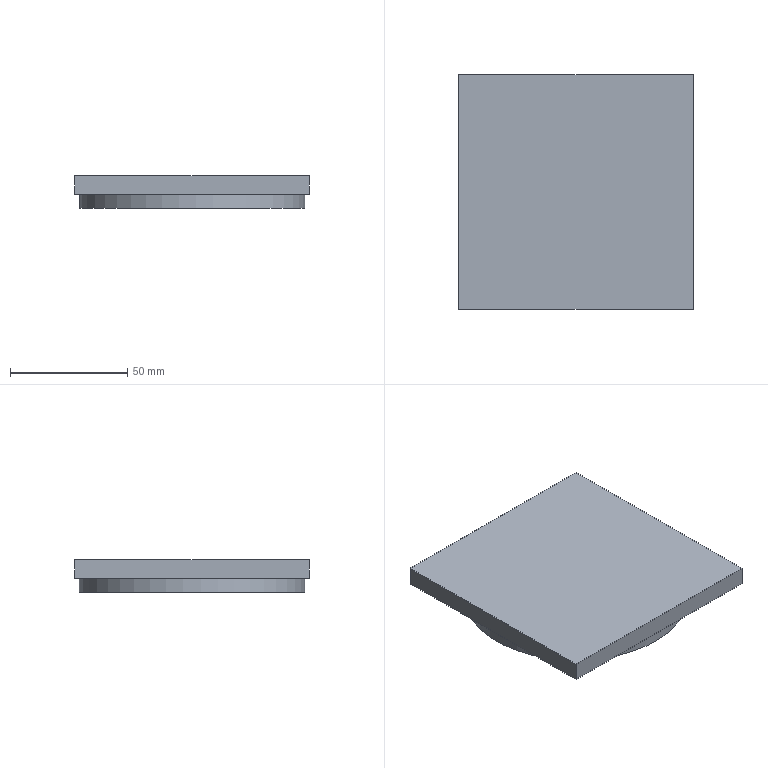NC program | NX | posted with a generic post | part box 100 x 100 x 14 mm
Whole program:
N10 G17 G21 G94 G90
(ADAPTIVE_MILLING_1_COPY , TOOL : D-12)
N12 T02 M6
N14 G54
N16 G17 G0 G90 X-1.135 Y5.279 S6000 M3
N18 G43 Z15. H2
N20 Z10.
N22 G94 G3 X-1.135 Y5.279 Z9.408 I1.135 J-5.279 F4000.
N24 X-1.135 Y5.279 Z8.816 I1.135 J-5.279
N26 X-1.135 Y5.279 Z8.223 I1.135 J-5.279
N28 X-1.135 Y5.279 Z7.631 I1.135 J-5.279
N30 X-1.135 Y5.279 Z7.039 I1.135 J-5.279
N32 X-1.135 Y5.279 Z6.447 I1.135 J-5.279
N34 X-1.135 Y5.279 Z5.854 I1.135 J-5.279
N36 X-1.135 Y5.279 Z5.262 I1.135 J-5.279
N38 X-1.135 Y5.279 Z4.67 I1.135 J-5.279
N40 X-1.135 Y5.279 Z4.078 I1.135 J-5.279
N42 X-1.135 Y5.279 Z3.485 I1.135 J-5.279
N44 X-1.135 Y5.279 Z2.893 I1.135 J-5.279
N46 X-1.135 Y5.279 Z2.301 I1.135 J-5.279
N48 X-1.135 Y5.279 Z1.709 I1.135 J-5.279
N50 X-1.135 Y5.279 Z1.116 I1.135 J-5.279
N52 X-1.135 Y5.279 Z0.524 I1.135 J-5.279
N54 X5.4 Y0. Z0.1 R-5.4
N56 X-3.183 Y-4.438 R-5.43
N58 X4.389 Y-3.32 R5.53
N60 X1.157 Y6.066 R5.7
N62 X0.068 Y-6.24 R-6.208
N64 X6.049 Y3.109 R6.703
N66 X-3.005 Y6.328 R6.76
N68 X-6.34 Y-3.048 R7.037
N70 X3.016 Y-6.393 R7.037
N72 X5.74 Y5.139 R7.442
N74 X-6.46 Y4.501 R7.722
N76 X2.461 Y-7.537 R7.902
N78 X0.478 Y8.702 R8.313
N80 X-6.031 Y-6.413 R8.751
N82 X6.609 Y-6.044 R9.029
N84 X0.165 Y9.64 R9.24
N86 X-7.235 Y-6.519 R9.676
N88 X6.659 Y-7.298 R9.937
N90 X1.171 Y10.532 R10.195
N92 X-9.22 Y-5.439 R10.635
N94 X5.817 Y-9.13 R10.861
N96 X1.397 Y11.498 R11.182
N98 X-10.325 Y-5.513 R11.627
N100 X5.527 Y-10.446 R11.852
N102 X2.228 Y12.392 R12.19
N104 X-11.976 Y-4.291 R12.627
N106 X4.618 Y-11.968 R12.843
N108 X6.27 Y12.045 R13.211
N110 X-11.992 Y6.715 R13.584
N112 X1.416 Y-13.769 R13.807
N114 X11.223 Y9.224 R14.234
N116 X-8.738 Y11.93 R14.517
N118 X-3.044 Y-14.576 R14.837
N120 X14.858 Y4.283 R15.27
N122 X-7.311 Y14.089 R15.534
N124 X-3.915 Y-15.492 R15.922
N126 X16.219 Y3.221 R16.345
N128 X-7.271 Y15.346 R16.635
N130 X-4.795 Y-16.41 R17.034
N132 X17.455 Y2.57 R17.467
N134 X-6.832 Y16.769 R17.753
N136 X-5.621 Y-17.339 R18.162
N138 X18.728 Y0.557 R18.576
N140 X-8.236 Y17.414 R18.896
N142 X-6.324 Y-18.319 R19.317
N144 X19.755 Y-1.884 R19.71
N146 X-7.623 Y18.946 R20.046
N148 X-7.754 Y-19.021 R20.476
N150 X20.749 Y-3.195 R20.874
N152 X-9.082 Y19.601 R21.222
N154 X-6.571 Y-20.711 R21.664
N156 X21.75 Y-4.243 R22.047
N158 X-8.523 Y21.136 R22.402
N160 X-8.396 Y-21.323 R22.855
N162 X22.554 Y-5.967 R23.222
N164 X-8.297 Y22.508 R23.59
N166 X-7.852 Y-22.808 R24.055
N168 X-5.596 Y-23.488 R42.922
N170 X-1.087 Y-24.123 R27.427
N172 X3.497 Y-23.893 R27.728
N174 X7.956 Y-22.799 R27.728
N176 X12.127 Y-20.881 R27.728
N178 X15.859 Y-18.209 R27.728
N180 X19.019 Y-14.878 R27.728
N182 X21.491 Y-11.01 R27.728
N184 X23.186 Y-6.744 R27.728
N186 X24.044 Y-2.234 R27.728
N188 G1 X24.147 Y0.062
N190 G3 X23.699 Y4.63 R27.728
N192 X22.394 Y9.032 R27.728
N194 X20.281 Y13.107 R27.728
N196 X17.434 Y16.708 R27.728
N198 X13.957 Y19.705 R27.728
N200 X9.975 Y21.991 R27.728
N202 X5.633 Y23.481 R27.728
N204 X1.087 Y24.123 R27.728
N206 X-3.497 Y23.893 R27.728
N208 X-7.956 Y22.799 R27.728
N210 X-12.127 Y20.881 R27.728
N212 X-15.859 Y18.209 R27.728
N214 X-19.019 Y14.878 R27.728
N216 X-21.491 Y11.01 R27.728
N218 X-23.186 Y6.744 R27.728
N220 X-24.044 Y2.234 R27.728
N222 G1 X-24.147 Y-0.062
N224 G3 X-23.699 Y-4.63 R27.728
N226 X-22.394 Y-9.032 R27.728
N228 X-20.281 Y-13.107 R27.728
N230 X-17.434 Y-16.708 R27.728
N232 X-13.957 Y-19.705 R27.728
N234 X-9.975 Y-21.991 R27.728
N236 X-5.633 Y-23.481 R27.801
N238 G1 X-5.449 Y-23.516
N240 G3 X-4.076 Y-22.727 R1.212
N242 G1 X-3.441 Y-20.914
N244 X-3.359 Y-20.678 Z0.106
N246 X-3.276 Y-20.442 Z0.125
N248 X-3.194 Y-20.206 Z0.157
N250 X-3.111 Y-19.97 Z0.201
N252 X-3.029 Y-19.734 Z0.259
N254 X-2.946 Y-19.498 Z0.33
N256 X-2.864 Y-19.262 Z0.416
N258 X-2.781 Y-19.026 Z0.517
N260 X-2.698 Y-18.791 Z0.635
N262 X-2.616 Y-18.555 Z0.77
N264 X-2.533 Y-18.319 Z0.924
N266 X-2.451 Y-18.083 Z1.1
N268 X-2.368 Y-17.847 Z1.3
N270 X-2.286 Y-17.611 Z1.529
N272 X-2.203 Y-17.375 Z1.793
N274 X-2.12 Y-17.139 Z2.1
N276 X-2.038 Y-16.903 Z2.466
N278 X-1.955 Y-16.667 Z2.921
N280 X-1.873 Y-16.431 Z3.539
N282 X-1.79 Y-16.195 Z5.1
N284 G0 Z15.
(ADAPTIVE_MILLING_1 , TOOL : D-12)
N286 X-65.106 Y-1.19
N288 Z3.1
N290 G1 X-64.957 Y-1.172 Z2.163
N292 X-64.808 Y-1.154 Z1.792
N294 X-64.659 Y-1.136 Z1.52
N296 X-64.51 Y-1.118 Z1.3
N298 X-64.361 Y-1.1 Z1.116
N300 X-64.212 Y-1.082 Z0.958
N302 X-64.063 Y-1.064 Z0.82
N304 X-63.914 Y-1.046 Z0.7
N306 X-63.765 Y-1.028 Z0.595
N308 X-63.616 Y-1.01 Z0.502
N310 X-63.468 Y-0.992 Z0.421
N312 X-63.319 Y-0.974 Z0.35
N314 X-63.17 Y-0.955 Z0.29
N316 X-63.021 Y-0.937 Z0.238
N318 X-62.872 Y-0.919 Z0.195
N320 X-62.723 Y-0.901 Z0.161
N322 X-62.574 Y-0.883 Z0.134
N324 X-62.425 Y-0.865 Z0.115
N326 X-62.276 Y-0.847 Z0.104
N328 X-62.127 Y-0.829 Z0.1
N330 X-60.02 Y-0.574
N332 G3 X-59.149 Y-0.031 R1.214
N334 X-58.37 Y1.824 R5.038
N336 X-57.71 Y7.174 R28.954
N338 X-57.503 Y20.054 R286.25
N340 G1 X-57.5 Y49.301
N342 G2 X-55.809 Y53.168 R6.003
N344 X-51.406 Y55.933 R10.785
N346 X-45.162 Y57.141 R25.43
N348 X-36.358 Y57.466 R117.958
N350 G1 X-24.358 Y57.499
N352 X49.339 Y57.498
N354 G2 X53.058 Y55.91 R5.988
N356 X55.822 Y51.71 R10.36
N358 X57.094 Y45.673 R23.648
N360 X57.464 Y36.496 R108.569
N362 G1 X57.499 Y24.496
N364 X57.496 Y-49.401
N366 G2 X55.771 Y-53.255 R6.049
N368 X51.345 Y-55.978 R10.69
N370 X45.095 Y-57.152 R25.981
N372 X36.29 Y-57.467 R121.773
N374 G1 X24.291 Y-57.499
N376 X-49.289 Y-57.498
N378 G2 X-53.173 Y-55.847 R5.994
N380 X-55.943 Y-51.451 R10.562
N382 X-57.143 Y-45.208 R25.353
N384 X-57.469 Y-36.028 R122.924
N386 G1 X-57.499 Y-24.403
N388 X-57.498 Y-4.791
N390 G2 X-57.03 Y-0.13 R39.338
N392 G3 X-56.094 Y12.827 R103.368
N394 X-56.001 Y23.989 R698.024
N396 G1 X-55.999 Y45.364
N398 G2 X-52.987 Y51.62 R8.625
N400 X-47.559 Y54.499 R14.146
N402 X-40.543 Y55.66 R33.747
N404 X-29.113 Y55.983 R175.201
N406 G1 X-18.8 Y55.999
N408 X45.362 Y55.996
N410 G2 X51.502 Y53.119 R8.6
N412 X54.451 Y47.726 R13.849
N414 X55.647 Y40.717 R32.691
N416 X55.982 Y29.286 R169.001
N418 G1 X55.999 Y18.974
N420 X55.996 Y-45.425
N422 G2 X52.972 Y-51.651 R8.593
N424 X47.713 Y-54.461 R13.965
N426 X40.885 Y-55.635 R32.52
N428 X30.58 Y-55.973 R149.383
N430 G1 X18.205 Y-55.999
N432 X-45.425 Y-55.996
N434 G2 X-51.527 Y-53.115 R8.518
N436 X-54.404 Y-47.905 R13.73
N438 X-55.618 Y-41.089 R31.501
N440 X-55.965 Y-31.347 R136.499
N442 G1 X-55.999 Y-18.972
N444 G2 X-55.972 Y-6.673 R849.673
N446 X-55.639 Y-1.998 R79.801
N448 G3 X-54.562 Y16.545 R177.328
N450 X-54.501 Y28.863 R760.801
N452 G2 X-54.48 Y42.475 R974.817
N454 X-50.588 Y50.076 R10.18
N456 X-44.563 Y53.015 R16.245
N458 X-37.162 Y54.156 R38.839
N460 X-25.918 Y54.478 R183.144
N462 G1 X-15.606 Y54.498
N464 X41.694 Y54.497
N466 G2 X48.33 Y52.324 R10.296
N468 X52.089 Y47.233 R12.945
N470 X53.839 Y40.351 R25.619
N472 X54.415 Y30.998 R88.487
N474 X54.498 Y15.436 R833.742
N476 G1 X54.497 Y-41.864
N478 G2 X50.195 Y-50.403 R10.301
N480 X44.058 Y-53.156 R17.136
N482 X36.453 Y-54.206 R42.51
N484 X24.833 Y-54.485 R214.703
N486 G1 X14.521 Y-54.499
N488 X-41.842 Y-54.497
N490 G2 X-50.302 Y-50.325 R10.263
N492 X-53.066 Y-44.407 R16.719
N494 X-54.194 Y-36.625 R41.002
N496 X-54.49 Y-23.506 R230.684
N498 X-54.461 Y-8.393 R826.864
N500 X-53.826 Y0.924 R163.894
N502 G3 X-53.051 Y18.971 R234.336
N504 X-53.001 Y31.301 R784.053
N506 G2 X-52.973 Y39.663 R420.928
N508 X-48.124 Y48.748 R11.35
N510 X-41.817 Y51.554 R18.29
N512 X-33.657 Y52.691 R44.415
N514 X-21.662 Y52.983 R220.176
N516 G1 X-11.349 Y52.998
N518 X38.638 Y52.996
N520 G2 X43.431 Y52.26 R13.701
N522 X49.148 Y47.553 R11.723
N524 X51.761 Y40.955 R19.774
N526 X52.753 Y32.586 R51.37
N528 X52.994 Y17.589 R325.731
N530 G1 X52.998 Y11.402
N532 X52.997 Y-38.586
N534 G2 X52.218 Y-43.558 R13.7
N536 X47.579 Y-49.139 R11.711
N538 X41.178 Y-51.716 R19.499
N540 X32.813 Y-52.741 R49.999
N542 X19.504 Y-52.991 R280.831
N544 G1 X11.254 Y-52.998
N546 X-38.734 Y-52.996
N548 G2 X-43.696 Y-52.168 R13.222
N550 X-49.29 Y-47.338 R11.861
N552 X-51.815 Y-40.716 R20.223
N554 X-52.775 Y-32.153 R54.626
N556 X-52.995 Y-17.531 R346.706
N558 X-52.794 Y-5.91 R189.127
N560 X-52.109 Y3.838 R840.735
N562 G3 X-51.524 Y23.45 R324.111
N564 G1 X-51.495 Y36.101
N566 G2 X-50.785 Y41.091 R15.796
N568 X-45.587 Y47.539 R12.403
N570 X-38.999 Y50.158 R20.666
N572 X-30.263 Y51.231 R52.212
N574 X-15.267 Y51.493 R309.56
N576 G1 X-9.079 Y51.497
N578 X35.471 Y51.496
N580 G2 X40.308 Y51.018 R18.887
N582 X47.325 Y45.913 R12.133
N584 X50.07 Y39.38 R19.925
N586 X51.188 Y31.027 R48.54
N588 X51.488 Y17.345 R253.87
N590 G1 X51.497 Y9.095
N592 X51.496 Y-35.642
N594 G2 X51.024 Y-40.293 R18.456
N596 X46.141 Y-47.177 R12.043
N598 X39.622 Y-50.013 R19.383
N600 X31.276 Y-51.172 R47.16
N602 X19.281 Y-51.479 R219.387
N604 G1 X8.969 Y-51.498
N606 X-35.581 Y-51.497
N608 G2 X-40.234 Y-51.042 R18.726
N610 X-47.261 Y-46.017 R12.12
N612 X-50.049 Y-39.471 R19.698
N614 X-51.182 Y-31.12 R48.244
N616 X-51.482 Y-18.75 R229.767
N618 X-51.023 Y-2.262 R194.687
N620 G3 X-50.02 Y25.318 R366.992
N622 G2 X-49.973 Y34.49 R753.692
N624 X-48.835 Y40.153 R15.159
N626 X-43.504 Y46.077 R13.178
N628 X-36.683 Y48.672 R22.06
N630 X-27.755 Y49.731 R55.843
N632 X-12.759 Y49.992 R318.189
N634 G1 X-6.572 Y49.997
N636 X32.728 Y49.996
N638 G2 X37.582 Y49.639 R24.755
N640 X45.724 Y44.056 R12.734
N642 X48.524 Y37.334 R20.668
N644 X49.683 Y28.609 R50.967
N646 X49.986 Y15.114 R254.68
N648 G1 X49.997 Y4.802
N650 X49.996 Y-32.811
N652 G2 X49.624 Y-37.663 R24.121
N654 X44.404 Y-45.488 R12.651
N656 X37.738 Y-48.425 R19.992
N658 X29.212 Y-49.645 R47.722
N660 X16.656 Y-49.978 R216.916
N662 G1 X6.344 Y-49.997
N664 X-32.956 Y-49.996
N666 G2 X-37.805 Y-49.593 R22.842
N668 X-45.542 Y-44.326 R12.662
N670 X-48.492 Y-37.462 R20.273
N672 X-49.686 Y-28.554 R50.383
N674 X-49.47 Y-1.758 R227.719
N676 G3 X-48.519 Y26.443 R411.942
N678 G2 X-48.424 Y33.184 R133.768
N680 X-46.698 Y39.456 R14.403
N682 X-41.156 Y44.806 R14.158
N684 X-33.918 Y47.3 R24.393
N686 X-24.414 Y48.277 R65.151
N688 X-7.729 Y48.494 R425.887
N690 G1 X-3.604 Y48.496
N692 X30.258 Y48.495
N694 G2 X35.488 Y48.132 R28.218
N696 X44.057 Y42.374 R13.169
N698 X46.957 Y35.482 R21.18
N700 X48.14 Y26.949 R50.242
N702 X48.477 Y14.205 R224.417
N704 G1 X48.496 Y3.893
N706 X48.495 Y-30.345
N708 G2 X48.152 Y-35.388 R27.979
N710 X42.316 Y-44.1 R13.174
N712 X35.418 Y-46.974 R21.319
N714 X26.509 Y-48.168 R51.615
N716 X11.889 Y-48.487 R269.101
N718 G1 X3.639 Y-48.497
N720 X-30.411 Y-48.495
N722 G2 X-35.637 Y-48.104 R26.794
N724 X-44.047 Y-42.388 R13.202
N726 X-46.954 Y-35.495 R21.104
N728 X-48.152 Y-26.775 R50.685
N730 X-48.074 Y-3.913 R198.191
N732 G3 X-47.151 Y16.578 R514.032
N734 X-46.992 Y29.636 R994.493
N736 G2 X-46.266 Y35.009 R20.408
N738 X-40.466 Y42.588 R13.651
N740 X-33.195 Y45.518 R22.477
N742 X-24.092 Y46.679 R55.237
N744 X-10.41 Y46.984 R266.627
N746 G1 X-0.097 Y46.996
N748 X27.765 Y46.995
N750 G2 X33.187 Y46.677 R33.812
N752 X42.619 Y40.417 R13.63
N754 X45.488 Y33.323 R22.371
N756 X46.671 Y24.223 R54.318
N758 X46.986 Y9.603 R275.688
N760 G1 X46.996 Y1.353
N762 X46.994 Y-28.01
N764 G2 X46.636 Y-33.428 R30.814
N766 X40.362 Y-42.657 R13.647
N768 X33.248 Y-45.506 R22.442
N770 X23.959 Y-46.686 R55.68
N772 X9.526 Y-46.986 R280.251
N774 G1 X1.276 Y-46.996
N776 X-27.899 Y-46.995
N778 G2 X-33.134 Y-46.687 R33.572
N780 X-42.604 Y-40.434 R13.676
N782 X-45.439 Y-33.52 R22.025
N784 X-46.669 Y-24.239 R53.477
N786 X-46.622 Y-5.31 R177.477
N788 G3 X-45.784 Y12.124 R845.3
N790 X-45.503 Y27.588 R888.308
N792 G2 X-44.758 Y33.147 R21.903
N794 X-38.853 Y40.95 R14.012
N796 X-31.784 Y43.888 R22.403
N798 X-22.506 Y45.146 R53.849
N800 X-7.699 Y45.484 R269.659
N802 G1 X2.614 Y45.495
N804 X25.601 Y45.494
N806 G2 X31.211 Y45.177 R36.735
N808 X41.071 Y38.672 R14.026
N810 X43.938 Y31.574 R22.76
N812 X45.148 Y22.477 R54.54
N814 X45.479 Y8.983 R249.15
N816 G1 X45.495 Y-1.33
N818 X45.494 Y-25.63
N820 G2 X45.173 Y-31.239 R36.221
N822 X38.782 Y-41. R14.009
N824 X31.69 Y-43.909 R22.517
N826 X22.41 Y-45.152 R54.613
N828 X8.915 Y-45.48 R253.527
N830 G1 X-1.397 Y-45.495
N832 X-25.697 Y-45.494
N834 G2 X-31.306 Y-45.16 R35.379
N836 X-40.916 Y-38.907 R13.991
N838 X-43.873 Y-31.831 R22.212
N840 X-45.138 Y-22.553 R52.764
N842 X-45.154 Y-6.622 R158.281
N844 G1 X-44.591 Y4.696
N846 G3 X-44.027 Y25.354 R596.954
N848 G2 X-43.365 Y30.927 R24.709
N850 X-37.062 Y39.47 R14.368
N852 X-29.959 Y42.369 R23.007
N854 X-20.681 Y43.631 R54.23
N856 X-6.437 Y43.98 R253.956
N858 G1 X3.875 Y43.995
N860 X23.488 Y43.993
N862 G2 X29.286 Y43.677 R39.986
N864 X39.585 Y36.874 R14.374
N866 X42.46 Y29.572 R23.691
N868 X43.667 Y20.097 R57.501
N870 X43.984 Y5.664 R279.301
N872 G1 X43.995 Y-4.648
N874 X43.993 Y-23.323
N876 G2 X43.672 Y-29.309 R40.482
N878 X36.981 Y-39.512 R14.311
N880 X29.706 Y-42.426 R23.3
N882 X20.234 Y-43.658 R56.465
N884 X5.802 Y-43.984 R271.693
N886 G1 X-4.51 Y-43.995
N888 X-23.56 Y-43.993
N890 G2 X-29.357 Y-43.662 R38.409
N892 X-39.462 Y-37.052 R14.314
N894 X-42.362 Y-29.971 R22.911
N896 X-43.641 Y-20.131 R53.762
N898 X-43.58 Y-5.511 R160.483
N900 G1 X-43.094 Y4.686
N902 G3 X-42.548 Y23.495 R661.769
N904 G2 X-41.839 Y29.251 R25.494
N906 X-35.354 Y37.945 R14.616
N908 X-28.084 Y40.874 R23.679
N910 X-18.801 Y42.124 R55.653
N912 X-5.495 Y42.475 R243.067
N914 G1 X6.88 Y42.495
N916 X21.43 Y42.493
N918 G2 X27.416 Y42.175 R42.357
N920 X38.054 Y35.167 R14.632
N922 X40.888 Y28.021 R23.783
N924 X42.128 Y18.74 R55.755
N926 X42.479 Y4.684 R253.775
N928 G1 X42.494 Y-5.629
N930 X42.493 Y-21.304
N932 G2 X42.191 Y-27.291 R43.889
N934 X35.417 Y-37.893 R14.583
N936 X27.927 Y-40.908 R23.743
N938 X18.83 Y-42.121 R56.289
N940 X4.774 Y-42.478 R249.584
N942 G1 X-5.538 Y-42.494
N944 X-21.401 Y-42.493
N946 G2 X-27.387 Y-42.177 R42.343
N948 X-38.11 Y-35.076 R14.69
N950 X-40.943 Y-27.765 R24.17
N952 X-42.126 Y-17.723 R56.089
N954 X-41.955 Y-3.104 R178.187
N956 G3 X-41.078 Y21.638 R775.325
N958 G2 X-40.327 Y27.577 R26.528
N960 X-33.754 Y36.377 R14.876
N962 X-26.122 Y39.41 R24.238
N964 X-16.65 Y40.638 R58.667
N966 X-1.843 Y40.981 R273.604
N968 G1 X8.47 Y40.994
N970 G2 X22.082 Y40.952 R743.127
N972 X27.83 Y40.199 R23.727
N974 X36.328 Y33.812 R14.773
N976 X39.306 Y26.551 R23.611
N978 X40.621 Y16.903 R55.981
N980 X40.981 Y1.909 R265.588
N982 G1 X40.994 Y-8.403
N984 G2 X40.949 Y-22.203 R707.735
N986 X40.114 Y-28.127 R22.934
N988 X33.679 Y-36.402 R14.804
N990 X26.195 Y-39.387 R24.217
N992 X16.537 Y-40.643 R58.363
N994 X1.731 Y-40.982 R273.535
N996 G1 X-8.582 Y-40.994
N998 G2 X-21.819 Y-40.961 R873.955
N1000 X-27.758 Y-40.218 R24.586
N1002 X-36.492 Y-33.547 R14.834
N1004 X-39.457 Y-25.852 R24.546
N1006 X-40.568 Y-15.99 R55.889
N1008 X-40.452 Y-3.619 R171.465
N1010 G1 X-40.096 Y4.67
N1012 G3 X-39.615 Y19.777 R860.665
N1014 G2 X-38.877 Y25.72 R28.243
N1016 X-32.28 Y34.747 R15.092
N1018 X-25.037 Y37.746 R23.761
N1020 X-15.768 Y39.072 R54.454
N1022 X-1.901 Y39.47 R228.047
N1024 G1 X10.474 Y39.494
N1026 G2 X20.898 Y39.426 R326.181
N1028 X26.981 Y38.419 R21.521
N1030 X35.051 Y31.757 R15.112
N1032 X37.885 Y24.434 R24.755
N1034 X39.148 Y14.589 R59.738
N1036 X39.477 Y0.532 R272.433
N1038 G1 X39.493 Y-9.78
N1040 G2 X39.431 Y-20.767 R375.09
N1042 X38.463 Y-26.858 R21.931
N1044 X32.323 Y-34.683 R14.923
N1046 X24.91 Y-37.766 R23.632
N1048 X15.639 Y-39.079 R54.822
N1050 X2.709 Y-39.465 R219.538
N1052 G1 X-9.666 Y-39.493
N1054 G2 X-20.278 Y-39.449 R457.959
N1056 X-26.21 Y-38.661 R24.325
N1058 X-34.929 Y-31.949 R15.021
N1060 X-37.896 Y-24.278 R24.379
N1062 X-39.01 Y-14.039 R55.753
N1064 X-38.842 Y-1.292 R190.329
N1066 G3 X-38.166 Y17.729 R888.584
N1068 G2 X-37.479 Y23.68 R31.037
N1070 X-30.18 Y33.518 R15.408
N1072 X-22.476 Y36.438 R25.648
N1074 X-12.624 Y37.655 R62.555
N1076 X2.183 Y37.981 R291.639
N1078 X17.933 Y37.962 R939.866
N1080 X23.887 Y37.318 R28.219
N1082 X33.333 Y30.432 R15.172
N1084 X36.361 Y22.783 R24.808
N1086 X37.612 Y13.314 R58.765
N1088 X37.976 Y-1.117 R258.762
N1090 X37.957 Y-18.105 R956.78
N1092 X37.23 Y-24.235 R26.917
N1094 X30.721 Y-33.14 R15.099
N1096 X23.107 Y-36.281 R24.169
N1098 X13.646 Y-37.59 R56.868
N1100 X-0.596 Y-37.973 R243.076
N1102 X-18.221 Y-37.954 R938.81
N1104 X-24.347 Y-37.199 R26.221
N1106 X-33.43 Y-30.262 R15.179
N1108 X-36.362 Y-22.574 R24.568
N1110 X-37.439 Y-12.333 R55.912
N1112 X-37.209 Y1.725 R219.523
N1114 G3 X-36.714 Y15.864 R871.115
N1116 G2 X-36.002 Y22.001 R32.207
N1118 X-28.74 Y31.895 R15.589
N1120 X-21.246 Y34.826 R25.178
N1122 X-11.592 Y36.108 R59.425
N1124 X2.839 Y36.475 R261.723
N1126 X16.714 Y36.444 R578.868
N1128 X22.835 Y35.647 R25.882
N1130 X31.769 Y28.873 R15.336
N1132 X34.776 Y21.41 R24.739
N1134 X36.083 Y11.949 R57.192
N1136 X36.474 Y-2.856 R251.079
N1138 X36.443 Y-16.731 R550.573
N1140 X35.64 Y-22.85 R25.49
N1142 X29.02 Y-31.669 R15.302
N1144 X21.408 Y-34.773 R24.528
N1146 X11.573 Y-36.108 R58.794
N1148 X-2.858 Y-36.474 R260.54
N1150 X-16.733 Y-36.443 R548.425
N1152 X-22.853 Y-35.641 R25.582
N1154 X-31.763 Y-28.858 R15.247
N1156 X-34.797 Y-21.003 R24.399
N1158 X-35.856 Y-10.947 R55.441
N1160 X-35.654 Y2.924 R226.723
N1162 X-35.187 Y15.497 R936.371
N1164 X-34.125 Y21.765 R24.876
N1166 X-27.37 Y30.236 R15.72
N1168 X-19.914 Y33.239 R24.996
N1170 X-10.268 Y34.578 R57.459
N1172 X4.724 Y34.975 R253.384
N1174 X15.598 Y34.917 R290.108
N1176 X21.876 Y33.927 R23.411
N1178 X30.243 Y27.277 R15.49
N1180 X33.29 Y19.651 R24.953
N1182 X34.581 Y10.185 R58.247
N1184 X34.968 Y-3.682 R239.89
N1186 X34.921 Y-15.494 R334.539
N1188 X34.013 Y-21.597 R23.999
N1190 X27.055 Y-30.377 R15.572
N1192 X19.579 Y-33.302 R25.294
N1194 X9.739 Y-34.609 R59.949
N1196 X-4.692 Y-34.974 R262.687
N1198 X-15.566 Y-34.918 R292.865
N1200 X-21.666 Y-33.994 R23.941
N1202 X-30.3 Y-27.131 R15.442
N1204 X-33.265 Y-19.268 R24.712
N1206 X-34.273 Y-9.583 R55.516
N1208 X-34.115 Y3.727 R222.505
N1210 X-33.706 Y14.191 R363.482
N1212 X-32.546 Y20.44 R24.008
N1214 X-25.477 Y28.911 R16.009
N1216 X-17.802 Y31.844 R26.002
N1218 X-7.77 Y33.126 R62.551
N1220 X7.412 Y33.478 R283.148
N1222 X15.283 Y33.329 R103.999
N1224 X21.653 Y31.886 R19.594
N1226 X28.945 Y25.315 R15.874
N1228 X31.825 Y17.811 R25.932
N1230 X33.111 Y7.967 R61.03
N1232 X33.477 Y-7.402 R277.667
N1234 X33.328 Y-15.274 R105.827
N1236 X31.736 Y-21.987 R19.385
N1238 X25.198 Y-29.015 R15.946
N1240 X17.503 Y-31.893 R26.34
N1242 X7.653 Y-33.13 R63.476
N1244 X-7.341 Y-33.477 R285.472
N1246 X-15.4 Y-33.318 R101.551
N1248 X-22.1 Y-31.677 R18.781
N1250 X-29.05 Y-25.049 R15.835
N1252 X-31.816 Y-17.102 R25.876
N1254 X-32.724 Y-6.842 R61.058
N1256 X-32.522 Y6.28 R275.144
N1258 X-32.118 Y13.955 R104.052
N1260 X-30.315 Y20.622 R19.64
N1262 X-23.634 Y27.557 R16.443
N1264 X-15.921 Y30.394 R26.896
N1266 X-5.696 Y31.646 R65.359
N1268 X11.923 Y31.913 R249.673
N1270 X18.22 Y31.031 R25.588
N1272 X27.132 Y24.206 R15.661
N1274 X30.218 Y16.596 R24.975
N1276 X31.589 Y6.577 R59.048
N1278 X31.903 Y-12.165 R236.891
N1280 X30.96 Y-18.452 R24.606
N1282 X24.019 Y-27.246 R15.794
N1284 X16.376 Y-30.267 R25.479
N1286 X6.725 Y-31.578 R59.767
N1288 X-12.017 Y-31.91 R239.505
N1290 X-18.309 Y-31.002 R24.956
N1292 X-27.234 Y-23.931 R15.55
N1294 X-30.106 Y-16.238 R24.709
N1296 X-31.123 Y-6.365 R56.125
N1298 X-30.79 Y10.877 R223.278
N1300 X-29.57 Y17.305 R24.505
N1302 X-22.297 Y25.913 R16.268
N1304 X-14.422 Y28.863 R26.954
N1306 X-4.198 Y30.134 R65.118
N1308 X10.796 Y30.374 R178.713
N1310 X17.251 Y29.317 R23.511
N1312 X25.608 Y22.641 R15.843
N1314 X28.744 Y14.844 R25.394
N1316 X30.08 Y5.008 R60.372
N1318 X30.376 Y-10.734 R177.145
N1320 X29.394 Y-17.014 R23.9
N1322 X22.524 Y-25.675 R15.796
N1324 X14.89 Y-28.726 R25.551
N1326 X4.868 Y-30.087 R60.149
N1328 X-10.687 Y-30.379 R178.867
N1330 X-16.789 Y-29.46 R24.365
N1332 X-25.672 Y-22.378 R15.579
N1334 X-28.537 Y-14.665 R24.748
N1336 X-29.544 Y-4.979 R56.101
N1338 X-29.307 Y9.451 R161.081
N1340 X-28.038 Y15.869 R23.849
N1342 X-20.872 Y24.326 R16.398
N1344 X-13.02 Y27.316 R26.655
N1346 X-2.801 Y28.618 R64.596
N1348 X9.38 Y28.835 R132.254
N1350 X15.827 Y27.74 R22.812
N1352 X24.138 Y20.997 R15.938
N1354 X27.202 Y13.376 R25.317
N1356 X28.552 Y3.73 R58.849
N1358 X28.834 Y-9.386 R131.986
N1360 X27.737 Y-15.833 R22.611
N1362 X21.137 Y-24.038 R15.813
N1364 X13.351 Y-27.201 R25.44
N1366 X3.706 Y-28.551 R59.028
N1368 X-9.411 Y-28.833 R130.946
N1370 X-15.677 Y-27.782 R22.674
N1372 X-24.184 Y-20.694 R15.587
N1374 X-27.037 Y-12.759 R25.342
N1376 X-27.984 Y-3.066 R59.162
N1378 X-27.781 Y8.364 R110.332
N1380 X-26.239 Y15.098 R21.951
N1382 X-19.188 Y22.9 R16.62
N1384 X-11.315 Y25.839 R27.171
N1386 X-1.093 Y27.12 R65.727
N1388 X8.464 Y27.252 R88.267
N1390 X15.221 Y25.841 R20.412
N1392 X22.914 Y18.947 R16.185
N1394 X25.865 Y11.037 R26.992
N1396 X27.13 Y0.814 R65.69
N1398 X27.245 Y-8.556 R85.422
N1400 X25.804 Y-15.307 R20.212
N1402 X19.167 Y-22.772 R16.107
N1404 X11.51 Y-25.749 R26.27
N1406 X1.298 Y-27.098 R62.061
N1408 X-8.633 Y-27.239 R85.641
N1410 X-15.027 Y-25.902 R19.946
N1412 X-22.726 Y-18.954 R15.706
N1414 X-25.5 Y-11.022 R25.787
N1416 X-26.433 Y-0.764 R62.282
N1418 X-26.169 Y7.851 R67.719
N1420 X-24.041 Y14.992 R19.088
N1422 X-17.077 Y21.709 R17.055
N1424 X-9.133 Y24.463 R28.844
N1426 X2.414 Y25.689 R70.334
N1428 X9.524 Y25.422 R39.112
N1430 X21.219 Y17.676 R16.017
N1432 X24.223 Y10.025 R26.12
N1434 X25.603 Y-0.559 R61.062
N1436 X25.579 Y-8.239 R53.322
N1438 X23.267 Y-15.696 R17.34
N1440 X16.568 Y-21.841 R16.919
N1442 X8.415 Y-24.565 R29.288
N1444 X-7.077 Y-25.666 R71.771
N1446 X-13.82 Y-24.201 R19.251
N1448 X-21.073 Y-17.554 R15.653
N1450 X-23.897 Y-9.635 R25.553
N1452 X-24.85 Y0.808 R58.573
N1454 X-24.381 Y8.094 R39.207
N1456 X-16.447 Y19.682 R16.545
N1458 X-8.615 Y22.726 R26.664
N1460 G3 X-5.694 Y23.469 R25.431
N1462 G1 X-3.437 Y23.904
N1464 X-1.149 Y24.123
N1466 G2 X4.524 Y24.139 R546.54
N1468 X11.167 Y23.102 R22.332
N1470 X19.42 Y16.557 R15.88
N1472 X22.633 Y8.798 R25.319
N1474 G1 X22.924 Y7.52
N1476 X23.172 Y6.804
N1478 X23.714 Y4.57
N1480 X24.041 Y2.296
N1482 G2 X24.039 Y-6.558 R64.902
N1484 X21.978 Y-13.711 R17.651
N1486 X15.3 Y-20.164 R16.675
N1488 X7.768 Y-22.86 R27.851
N1490 G1 X5.694 Y-23.469
N1492 X3.437 Y-23.904
N1494 X1.149 Y-24.123
N1496 G2 X-4.524 Y-24.137 R504.871
N1498 X-10.806 Y-23.195 R22.153
N1500 X-19.257 Y-16.423 R15.357
N1502 X-21.812 Y-10.307 R23.051
N1504 G1 X-22.42 Y-8.976
N1506 X-23.172 Y-6.804
N1508 X-23.714 Y-4.57
N1510 X-24.041 Y-2.296
N1512 X-24.15 Y0.
N1514 X-24.041 Y2.296
N1516 X-23.714 Y4.57
N1518 G2 X-22.312 Y9.48 R37.371
N1520 X-19.089 Y14.779 R17.08
N1522 X-17.478 Y16.665 R95.699
N1524 G1 X-15.815 Y18.251
N1526 X-14.008 Y19.672
N1528 X-12.075 Y20.915
N1530 X-10.032 Y21.968
N1532 X-7.899 Y22.822
N1534 X-5.694 Y23.469
N1536 X-3.437 Y23.904
N1538 X-1.149 Y24.123
N1540 X1.149
N1542 X3.437 Y23.904
N1544 X5.694 Y23.469
N1546 X7.899 Y22.822
N1548 X10.032 Y21.968
N1550 X12.075 Y20.915
N1552 X14.008 Y19.672
N1554 X15.815 Y18.251
N1556 X17.478 Y16.665
N1558 X18.983 Y14.929
N1560 X20.316 Y13.056
N1562 X21.465 Y11.066
N1564 X22.42 Y8.976
N1566 X23.172 Y6.804
N1568 X23.714 Y4.57
N1570 X24.041 Y2.296
N1572 X24.15 Y0.
N1574 X24.041 Y-2.296
N1576 X23.714 Y-4.57
N1578 X23.172 Y-6.804
N1580 X22.42 Y-8.976
N1582 X21.465 Y-11.066
N1584 X20.316 Y-13.056
N1586 X18.983 Y-14.929
N1588 X17.478 Y-16.665
N1590 X15.815 Y-18.251
N1592 X14.008 Y-19.672
N1594 X12.075 Y-20.915
N1596 X10.032 Y-21.968
N1598 G2 X7.719 Y-22.875 R75.73
N1600 G1 X5.694 Y-23.469
N1602 X3.437 Y-23.904
N1604 X1.149 Y-24.123
N1606 X-1.149
N1608 X-3.437 Y-23.904
N1610 X-5.694 Y-23.469
N1612 X-7.899 Y-22.822
N1614 X-10.032 Y-21.968
N1616 X-12.075 Y-20.915
N1618 X-14.008 Y-19.672
N1620 X-15.815 Y-18.251
N1622 X-17.478 Y-16.665
N1624 X-18.983 Y-14.929
N1626 X-20.316 Y-13.056
N1628 X-21.465 Y-11.066
N1630 X-22.42 Y-8.976
N1632 X-23.172 Y-6.804
N1634 X-23.714 Y-4.57
N1636 X-24.041 Y-2.296
N1638 X-24.15 Y0.
N1640 X-24.041 Y2.296
N1642 X-23.714 Y4.57
N1644 X-23.172 Y6.804
N1646 X-22.42 Y8.976
N1648 X-21.465 Y11.066
N1650 X-20.316 Y13.056
N1652 X-19.011 Y14.889
N1654 G3 X-19.063 Y16.363 R1.212
N1656 G1 X-20.311 Y17.876
N1658 X-20.406 Y17.992 Z0.104
N1660 X-20.502 Y18.108 Z0.115
N1662 X-20.597 Y18.223 Z0.134
N1664 X-20.693 Y18.339 Z0.161
N1666 X-20.788 Y18.455 Z0.195
N1668 X-20.884 Y18.57 Z0.238
N1670 X-20.979 Y18.686 Z0.29
N1672 X-21.075 Y18.802 Z0.35
N1674 X-21.17 Y18.918 Z0.421
N1676 X-21.265 Y19.033 Z0.502
N1678 X-21.361 Y19.149 Z0.595
N1680 X-21.456 Y19.265 Z0.7
N1682 X-21.552 Y19.38 Z0.82
N1684 X-21.647 Y19.496 Z0.958
N1686 X-21.743 Y19.612 Z1.116
N1688 X-21.838 Y19.728 Z1.3
N1690 X-21.933 Y19.843 Z1.52
N1692 X-22.029 Y19.959 Z1.792
N1694 X-22.124 Y20.075 Z2.163
N1696 X-22.22 Y20.19 Z3.1
N1698 G0 Z15.
N1700 M5
(FLOOR_FACING_1 , TOOL : FACEMILL-60)
N1702 T01 M6
N1704 G54
N1706 G17 G0 G90 X-90.12 Y21. S4000 M3
N1708 G43 Z14. H1
N1710 Z3.
N1712 G94 G1 Z0. F500.
N1714 X-75.12
N1716 X75.12
N1718 X90.12
N1720 Z3.
N1722 G0 Z14.
N1724 X-89.216 Y-24.
N1726 Z3.
N1728 G1 Z0.
N1730 X-74.216
N1732 X74.216
N1734 X89.216
N1736 Z3.
N1738 G0 Z14.
N1740 M5
(PLANAR_MILL_2_COPY_1 , TOOL : SPOTDRILL-D8)
N1742 T04 M6
N1744 G54
N1746 G17 G0 G90 X-18.542 Y2. S3000 M3
N1748 G43 Z10. H4
N1750 Z1.5
N1752 G94 G1 Z-1.5 F1500.
N1754 X-20.65
N1756 G3 X-22.65 Y0. R2.
N1758 X0. Y-22.65 R22.65
N1760 X-22.65 Y0. R-22.65
N1762 X-20.65 Y-2. R2.
N1764 G1 X-18.542
N1766 Z1.5
N1768 G0 Z10.
(PLANAR_MILL_2_COPY_1_COPY , TOOL : SPOTDRILL-D8)
N1770 X53.463 Y2.
N1772 Z1.5
N1774 G1 Z-1.5
N1776 X51.5
N1778 G3 X49.5 Y0. R2.
N1780 G2 X0. Y-49.5 R49.5
N1782 X49.5 Y0. R-49.5
N1784 G3 X51.5 Y-2. R2.
N1786 G1 X53.463
N1788 Z1.5
N1790 G0 Z10.
N1792 M5
N1794 M2